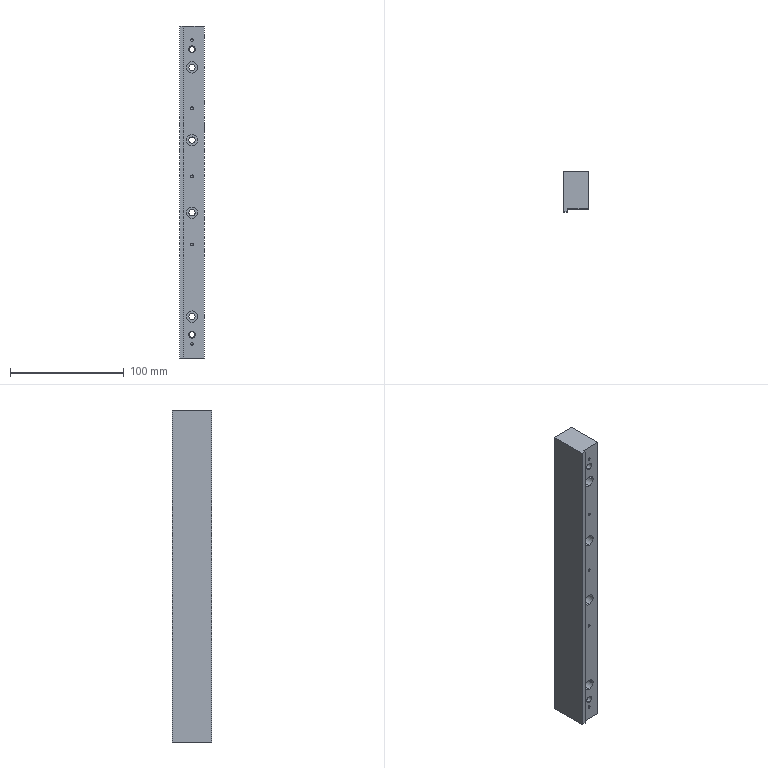Part | SolidWorks | features BaseBody 1 | 1 solid | 82 faces | box 22 x 35 x 292.5 mm | volume 202121 mm3 | cylinder 48 | cone 20 | plane 14 | commonest cylinder face diameters 2.5 x24 5.5 x8 10 x8 5 x4 6 x4